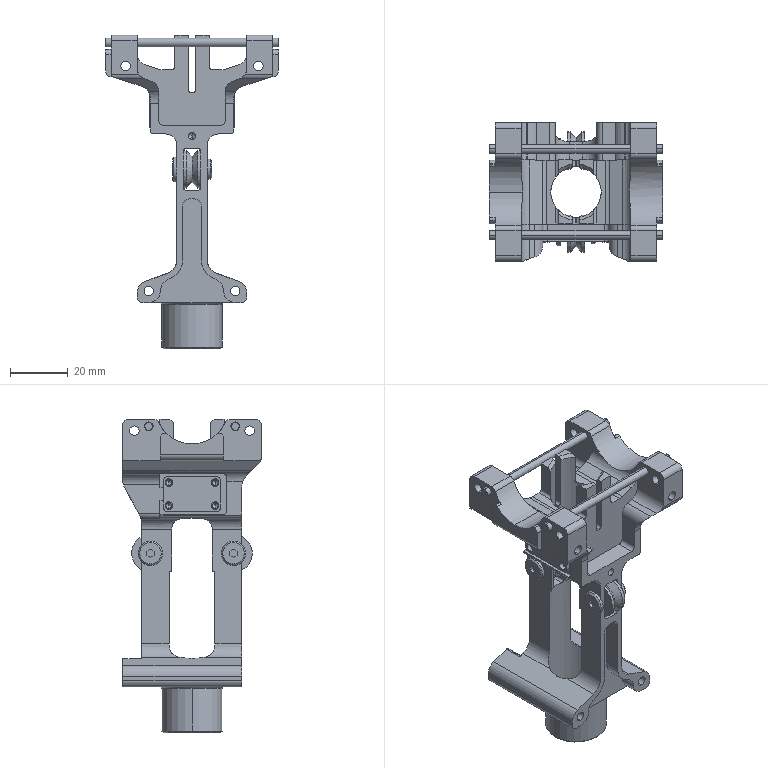Part | SolidWorks | features CompositeCurve 2 | 17 solids | 552 faces | box 60 x 48 x 108.75 mm | volume 39263 mm3 | cylinder 248 | plane 216 | cone 74 | torus 8 | sphere 4 | spline 2 | commonest cylinder face diameters 2 x41 4 x30 3 x22 8 x18 2.05 x16 2.7 x16